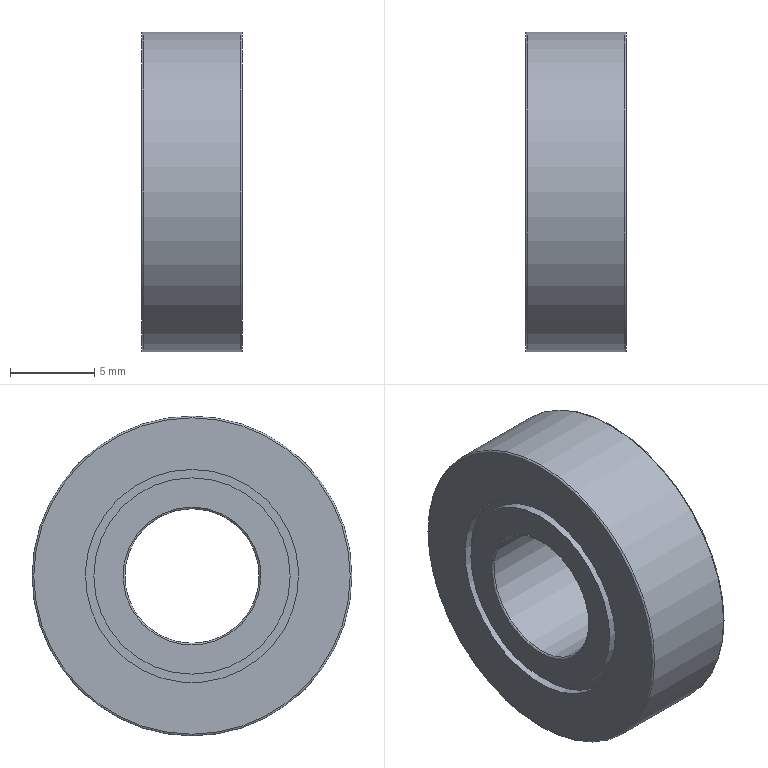Part | NX | 1 solid | 16 faces | box 6 x 19 x 19 mm | volume 1380 mm3 | plane 6 | cylinder 6 | torus 4 | commonest cylinder face diameters 11.667 x2 12.667 x2 8 x1 19 x1
STEP:
#1=CARTESIAN_POINT('',(-3.,0.,9.4));
#2=VERTEX_POINT('',#1);
#3=CARTESIAN_POINT('',(-3.,0.,0.));
#4=DIRECTION('',(-1.,0.,0.));
#5=DIRECTION('',(0.,0.,1.));
#6=AXIS2_PLACEMENT_3D('',#3,#4,#5);
#7=CIRCLE('',#6,9.4);
#8=EDGE_CURVE('',#2,#2,#7,.T.);
#9=ORIENTED_EDGE('',*,*,#8,.F.);
#10=EDGE_LOOP('',(#9));
#11=FACE_BOUND('',#10,.T.);
#12=CARTESIAN_POINT('',(-2.9,0.,9.5));
#13=VERTEX_POINT('',#12);
#14=CARTESIAN_POINT('',(-2.9,0.,0.));
#15=DIRECTION('',(-1.,0.,0.));
#16=DIRECTION('',(0.,0.,1.));
#17=AXIS2_PLACEMENT_3D('',#14,#15,#16);
#18=CIRCLE('',#17,9.5);
#19=EDGE_CURVE('',#13,#13,#18,.T.);
#20=ORIENTED_EDGE('',*,*,#19,.T.);
#21=EDGE_LOOP('',(#20));
#22=FACE_BOUND('',#21,.T.);
#23=CARTESIAN_POINT('',(-2.9,0.,0.));
#24=DIRECTION('',(-1.,0.,0.));
#25=DIRECTION('',(0.,0.,1.));
#26=AXIS2_PLACEMENT_3D('',#23,#24,#25);
#27=TOROIDAL_SURFACE('',#26,9.4,0.1);
#28=ADVANCED_FACE('',(#11,#22),#27,.T.);
#29=CARTESIAN_POINT('',(-3.,0.,6.333));
#30=VERTEX_POINT('',#29);
#31=CARTESIAN_POINT('',(-3.,0.,0.));
#32=DIRECTION('',(-1.,0.,0.));
#33=DIRECTION('',(0.,0.,1.));
#34=AXIS2_PLACEMENT_3D('',#31,#32,#33);
#35=CIRCLE('',#34,6.333);
#36=EDGE_CURVE('',#30,#30,#35,.T.);
#37=ORIENTED_EDGE('',*,*,#36,.F.);
#38=EDGE_LOOP('',(#37));
#39=FACE_BOUND('',#38,.T.);
#40=ORIENTED_EDGE('',*,*,#8,.T.);
#41=EDGE_LOOP('',(#40));
#42=FACE_BOUND('',#41,.T.);
#43=CARTESIAN_POINT('',(-3.,9.4,0.));
#44=DIRECTION('',(1.,0.,0.));
#45=DIRECTION('',(0.,0.,-1.));
#46=AXIS2_PLACEMENT_3D('',#43,#44,#45);
#47=PLANE('',#46);
#48=ADVANCED_FACE('',(#39,#42),#47,.F.);
#49=CARTESIAN_POINT('',(-2.5,0.,6.333));
#50=VERTEX_POINT('',#49);
#51=CARTESIAN_POINT('',(-2.5,0.,0.));
#52=DIRECTION('',(-1.,0.,0.));
#53=DIRECTION('',(0.,0.,1.));
#54=AXIS2_PLACEMENT_3D('',#51,#52,#53);
#55=CIRCLE('',#54,6.333);
#56=EDGE_CURVE('',#50,#50,#55,.T.);
#57=ORIENTED_EDGE('',*,*,#56,.F.);
#58=EDGE_LOOP('',(#57));
#59=FACE_BOUND('',#58,.T.);
#60=ORIENTED_EDGE('',*,*,#36,.T.);
#61=EDGE_LOOP('',(#60));
#62=FACE_BOUND('',#61,.T.);
#63=CARTESIAN_POINT('',(3.,0.,0.));
#64=DIRECTION('',(-1.,0.,0.));
#65=DIRECTION('',(0.,0.,1.));
#66=AXIS2_PLACEMENT_3D('',#63,#64,#65);
#67=CYLINDRICAL_SURFACE('',#66,6.333);
#68=ADVANCED_FACE('',(#59,#62),#67,.F.);
#69=CARTESIAN_POINT('',(-2.5,0.,5.833));
#70=VERTEX_POINT('',#69);
#71=CARTESIAN_POINT('',(-2.5,0.,0.));
#72=DIRECTION('',(-1.,0.,0.));
#73=DIRECTION('',(0.,0.,1.));
#74=AXIS2_PLACEMENT_3D('',#71,#72,#73);
#75=CIRCLE('',#74,5.833);
#76=EDGE_CURVE('',#70,#70,#75,.T.);
#77=ORIENTED_EDGE('',*,*,#76,.F.);
#78=EDGE_LOOP('',(#77));
#79=FACE_BOUND('',#78,.T.);
#80=ORIENTED_EDGE('',*,*,#56,.T.);
#81=EDGE_LOOP('',(#80));
#82=FACE_BOUND('',#81,.T.);
#83=CARTESIAN_POINT('',(-2.5,6.333,0.));
#84=DIRECTION('',(1.,0.,0.));
#85=DIRECTION('',(0.,0.,-1.));
#86=AXIS2_PLACEMENT_3D('',#83,#84,#85);
#87=PLANE('',#86);
#88=ADVANCED_FACE('',(#79,#82),#87,.F.);
#89=CARTESIAN_POINT('',(-3.,0.,5.833));
#90=VERTEX_POINT('',#89);
#91=CARTESIAN_POINT('',(-3.,0.,0.));
#92=DIRECTION('',(-1.,0.,0.));
#93=DIRECTION('',(0.,0.,1.));
#94=AXIS2_PLACEMENT_3D('',#91,#92,#93);
#95=CIRCLE('',#94,5.833);
#96=EDGE_CURVE('',#90,#90,#95,.T.);
#97=ORIENTED_EDGE('',*,*,#96,.F.);
#98=EDGE_LOOP('',(#97));
#99=FACE_BOUND('',#98,.T.);
#100=ORIENTED_EDGE('',*,*,#76,.T.);
#101=EDGE_LOOP('',(#100));
#102=FACE_BOUND('',#101,.T.);
#103=CARTESIAN_POINT('',(3.,0.,0.));
#104=DIRECTION('',(-1.,0.,0.));
#105=DIRECTION('',(0.,0.,1.));
#106=AXIS2_PLACEMENT_3D('',#103,#104,#105);
#107=CYLINDRICAL_SURFACE('',#106,5.833);
#108=ADVANCED_FACE('',(#99,#102),#107,.T.);
#109=CARTESIAN_POINT('',(-3.,0.,4.1));
#110=VERTEX_POINT('',#109);
#111=CARTESIAN_POINT('',(-3.,0.,0.));
#112=DIRECTION('',(-1.,0.,0.));
#113=DIRECTION('',(0.,0.,1.));
#114=AXIS2_PLACEMENT_3D('',#111,#112,#113);
#115=CIRCLE('',#114,4.1);
#116=EDGE_CURVE('',#110,#110,#115,.T.);
#117=ORIENTED_EDGE('',*,*,#116,.F.);
#118=EDGE_LOOP('',(#117));
#119=FACE_BOUND('',#118,.T.);
#120=ORIENTED_EDGE('',*,*,#96,.T.);
#121=EDGE_LOOP('',(#120));
#122=FACE_BOUND('',#121,.T.);
#123=CARTESIAN_POINT('',(-3.,5.833,0.));
#124=DIRECTION('',(1.,0.,0.));
#125=DIRECTION('',(0.,0.,-1.));
#126=AXIS2_PLACEMENT_3D('',#123,#124,#125);
#127=PLANE('',#126);
#128=ADVANCED_FACE('',(#119,#122),#127,.F.);
#129=CARTESIAN_POINT('',(-2.9,0.,4.));
#130=VERTEX_POINT('',#129);
#131=CARTESIAN_POINT('',(-2.9,0.,0.));
#132=DIRECTION('',(-1.,0.,0.));
#133=DIRECTION('',(0.,0.,1.));
#134=AXIS2_PLACEMENT_3D('',#131,#132,#133);
#135=CIRCLE('',#134,4.);
#136=EDGE_CURVE('',#130,#130,#135,.T.);
#137=ORIENTED_EDGE('',*,*,#136,.F.);
#138=EDGE_LOOP('',(#137));
#139=FACE_BOUND('',#138,.T.);
#140=ORIENTED_EDGE('',*,*,#116,.T.);
#141=EDGE_LOOP('',(#140));
#142=FACE_BOUND('',#141,.T.);
#143=CARTESIAN_POINT('',(-2.9,0.,0.));
#144=DIRECTION('',(-1.,0.,0.));
#145=DIRECTION('',(0.,0.,1.));
#146=AXIS2_PLACEMENT_3D('',#143,#144,#145);
#147=TOROIDAL_SURFACE('',#146,4.1,0.1);
#148=ADVANCED_FACE('',(#139,#142),#147,.T.);
#149=CARTESIAN_POINT('',(2.9,0.,4.));
#150=VERTEX_POINT('',#149);
#151=CARTESIAN_POINT('',(2.9,0.,0.));
#152=DIRECTION('',(-1.,0.,0.));
#153=DIRECTION('',(0.,0.,1.));
#154=AXIS2_PLACEMENT_3D('',#151,#152,#153);
#155=CIRCLE('',#154,4.);
#156=EDGE_CURVE('',#150,#150,#155,.T.);
#157=ORIENTED_EDGE('',*,*,#156,.F.);
#158=EDGE_LOOP('',(#157));
#159=FACE_BOUND('',#158,.T.);
#160=ORIENTED_EDGE('',*,*,#136,.T.);
#161=EDGE_LOOP('',(#160));
#162=FACE_BOUND('',#161,.T.);
#163=CARTESIAN_POINT('',(3.,0.,0.));
#164=DIRECTION('',(-1.,0.,0.));
#165=DIRECTION('',(0.,0.,1.));
#166=AXIS2_PLACEMENT_3D('',#163,#164,#165);
#167=CYLINDRICAL_SURFACE('',#166,4.);
#168=ADVANCED_FACE('',(#159,#162),#167,.F.);
#169=CARTESIAN_POINT('',(3.,0.,4.1));
#170=VERTEX_POINT('',#169);
#171=CARTESIAN_POINT('',(3.,0.,0.));
#172=DIRECTION('',(-1.,0.,0.));
#173=DIRECTION('',(0.,0.,1.));
#174=AXIS2_PLACEMENT_3D('',#171,#172,#173);
#175=CIRCLE('',#174,4.1);
#176=EDGE_CURVE('',#170,#170,#175,.T.);
#177=ORIENTED_EDGE('',*,*,#176,.F.);
#178=EDGE_LOOP('',(#177));
#179=FACE_BOUND('',#178,.T.);
#180=ORIENTED_EDGE('',*,*,#156,.T.);
#181=EDGE_LOOP('',(#180));
#182=FACE_BOUND('',#181,.T.);
#183=CARTESIAN_POINT('',(2.9,0.,0.));
#184=DIRECTION('',(-1.,0.,0.));
#185=DIRECTION('',(0.,0.,1.));
#186=AXIS2_PLACEMENT_3D('',#183,#184,#185);
#187=TOROIDAL_SURFACE('',#186,4.1,0.1);
#188=ADVANCED_FACE('',(#179,#182),#187,.T.);
#189=CARTESIAN_POINT('',(3.,0.,5.833));
#190=VERTEX_POINT('',#189);
#191=CARTESIAN_POINT('',(3.,0.,0.));
#192=DIRECTION('',(-1.,0.,0.));
#193=DIRECTION('',(0.,0.,1.));
#194=AXIS2_PLACEMENT_3D('',#191,#192,#193);
#195=CIRCLE('',#194,5.833);
#196=EDGE_CURVE('',#190,#190,#195,.T.);
#197=ORIENTED_EDGE('',*,*,#196,.F.);
#198=EDGE_LOOP('',(#197));
#199=FACE_BOUND('',#198,.T.);
#200=ORIENTED_EDGE('',*,*,#176,.T.);
#201=EDGE_LOOP('',(#200));
#202=FACE_BOUND('',#201,.T.);
#203=CARTESIAN_POINT('',(3.,4.1,0.));
#204=DIRECTION('',(-1.,0.,0.));
#205=DIRECTION('',(0.,0.,1.));
#206=AXIS2_PLACEMENT_3D('',#203,#204,#205);
#207=PLANE('',#206);
#208=ADVANCED_FACE('',(#199,#202),#207,.F.);
#209=CARTESIAN_POINT('',(2.5,0.,5.833));
#210=VERTEX_POINT('',#209);
#211=CARTESIAN_POINT('',(2.5,0.,0.));
#212=DIRECTION('',(-1.,0.,0.));
#213=DIRECTION('',(0.,0.,1.));
#214=AXIS2_PLACEMENT_3D('',#211,#212,#213);
#215=CIRCLE('',#214,5.833);
#216=EDGE_CURVE('',#210,#210,#215,.T.);
#217=ORIENTED_EDGE('',*,*,#216,.F.);
#218=EDGE_LOOP('',(#217));
#219=FACE_BOUND('',#218,.T.);
#220=ORIENTED_EDGE('',*,*,#196,.T.);
#221=EDGE_LOOP('',(#220));
#222=FACE_BOUND('',#221,.T.);
#223=CARTESIAN_POINT('',(3.,0.,0.));
#224=DIRECTION('',(-1.,0.,0.));
#225=DIRECTION('',(0.,0.,1.));
#226=AXIS2_PLACEMENT_3D('',#223,#224,#225);
#227=CYLINDRICAL_SURFACE('',#226,5.833);
#228=ADVANCED_FACE('',(#219,#222),#227,.T.);
#229=CARTESIAN_POINT('',(2.5,0.,6.333));
#230=VERTEX_POINT('',#229);
#231=CARTESIAN_POINT('',(2.5,0.,0.));
#232=DIRECTION('',(-1.,0.,0.));
#233=DIRECTION('',(0.,0.,1.));
#234=AXIS2_PLACEMENT_3D('',#231,#232,#233);
#235=CIRCLE('',#234,6.333);
#236=EDGE_CURVE('',#230,#230,#235,.T.);
#237=ORIENTED_EDGE('',*,*,#236,.F.);
#238=EDGE_LOOP('',(#237));
#239=FACE_BOUND('',#238,.T.);
#240=ORIENTED_EDGE('',*,*,#216,.T.);
#241=EDGE_LOOP('',(#240));
#242=FACE_BOUND('',#241,.T.);
#243=CARTESIAN_POINT('',(2.5,5.833,0.));
#244=DIRECTION('',(-1.,0.,0.));
#245=DIRECTION('',(0.,0.,1.));
#246=AXIS2_PLACEMENT_3D('',#243,#244,#245);
#247=PLANE('',#246);
#248=ADVANCED_FACE('',(#239,#242),#247,.F.);
#249=CARTESIAN_POINT('',(3.,0.,6.333));
#250=VERTEX_POINT('',#249);
#251=CARTESIAN_POINT('',(3.,0.,0.));
#252=DIRECTION('',(-1.,0.,0.));
#253=DIRECTION('',(0.,0.,1.));
#254=AXIS2_PLACEMENT_3D('',#251,#252,#253);
#255=CIRCLE('',#254,6.333);
#256=EDGE_CURVE('',#250,#250,#255,.T.);
#257=ORIENTED_EDGE('',*,*,#256,.F.);
#258=EDGE_LOOP('',(#257));
#259=FACE_BOUND('',#258,.T.);
#260=ORIENTED_EDGE('',*,*,#236,.T.);
#261=EDGE_LOOP('',(#260));
#262=FACE_BOUND('',#261,.T.);
#263=CARTESIAN_POINT('',(3.,0.,0.));
#264=DIRECTION('',(-1.,0.,0.));
#265=DIRECTION('',(0.,0.,1.));
#266=AXIS2_PLACEMENT_3D('',#263,#264,#265);
#267=CYLINDRICAL_SURFACE('',#266,6.333);
#268=ADVANCED_FACE('',(#259,#262),#267,.F.);
#269=CARTESIAN_POINT('',(3.,0.,9.4));
#270=VERTEX_POINT('',#269);
#271=CARTESIAN_POINT('',(3.,0.,0.));
#272=DIRECTION('',(-1.,0.,0.));
#273=DIRECTION('',(0.,0.,1.));
#274=AXIS2_PLACEMENT_3D('',#271,#272,#273);
#275=CIRCLE('',#274,9.4);
#276=EDGE_CURVE('',#270,#270,#275,.T.);
#277=ORIENTED_EDGE('',*,*,#276,.F.);
#278=EDGE_LOOP('',(#277));
#279=FACE_BOUND('',#278,.T.);
#280=ORIENTED_EDGE('',*,*,#256,.T.);
#281=EDGE_LOOP('',(#280));
#282=FACE_BOUND('',#281,.T.);
#283=CARTESIAN_POINT('',(3.,6.333,0.));
#284=DIRECTION('',(-1.,0.,0.));
#285=DIRECTION('',(0.,0.,1.));
#286=AXIS2_PLACEMENT_3D('',#283,#284,#285);
#287=PLANE('',#286);
#288=ADVANCED_FACE('',(#279,#282),#287,.F.);
#289=CARTESIAN_POINT('',(2.9,0.,9.5));
#290=VERTEX_POINT('',#289);
#291=CARTESIAN_POINT('',(2.9,0.,0.));
#292=DIRECTION('',(-1.,0.,0.));
#293=DIRECTION('',(0.,0.,1.));
#294=AXIS2_PLACEMENT_3D('',#291,#292,#293);
#295=CIRCLE('',#294,9.5);
#296=EDGE_CURVE('',#290,#290,#295,.T.);
#297=ORIENTED_EDGE('',*,*,#296,.F.);
#298=EDGE_LOOP('',(#297));
#299=FACE_BOUND('',#298,.T.);
#300=ORIENTED_EDGE('',*,*,#276,.T.);
#301=EDGE_LOOP('',(#300));
#302=FACE_BOUND('',#301,.T.);
#303=CARTESIAN_POINT('',(2.9,0.,0.));
#304=DIRECTION('',(-1.,0.,0.));
#305=DIRECTION('',(0.,0.,1.));
#306=AXIS2_PLACEMENT_3D('',#303,#304,#305);
#307=TOROIDAL_SURFACE('',#306,9.4,0.1);
#308=ADVANCED_FACE('',(#299,#302),#307,.T.);
#309=ORIENTED_EDGE('',*,*,#19,.F.);
#310=EDGE_LOOP('',(#309));
#311=FACE_BOUND('',#310,.T.);
#312=ORIENTED_EDGE('',*,*,#296,.T.);
#313=EDGE_LOOP('',(#312));
#314=FACE_BOUND('',#313,.T.);
#315=CARTESIAN_POINT('',(3.,0.,0.));
#316=DIRECTION('',(-1.,0.,0.));
#317=DIRECTION('',(0.,0.,1.));
#318=AXIS2_PLACEMENT_3D('',#315,#316,#317);
#319=CYLINDRICAL_SURFACE('',#318,9.5);
#320=ADVANCED_FACE('',(#311,#314),#319,.T.);
#321=CLOSED_SHELL('',(#28,#48,#68,#88,#108,#128,#148,#168,#188,#208,#228,#248,#268,#288,#308,#320));
#322=MANIFOLD_SOLID_BREP('',#321);
#323=(LENGTH_UNIT()NAMED_UNIT(*)SI_UNIT(.MILLI.,.METRE.));
#324=UNCERTAINTY_MEASURE_WITH_UNIT(LENGTH_MEASURE(0.00001),#323,'','');
#325=(NAMED_UNIT(*)PLANE_ANGLE_UNIT()SI_UNIT($,.RADIAN.));
#326=(NAMED_UNIT(*)SI_UNIT($,.STERADIAN.)SOLID_ANGLE_UNIT());
#327=(GEOMETRIC_REPRESENTATION_CONTEXT(3)GLOBAL_UNCERTAINTY_ASSIGNED_CONTEXT((#324))GLOBAL_UNIT_ASSIGNED_CONTEXT((#323,#325,#326))REPRESENTATION_CONTEXT('',''));
#328=ADVANCED_BREP_SHAPE_REPRESENTATION('',(#322),#327);